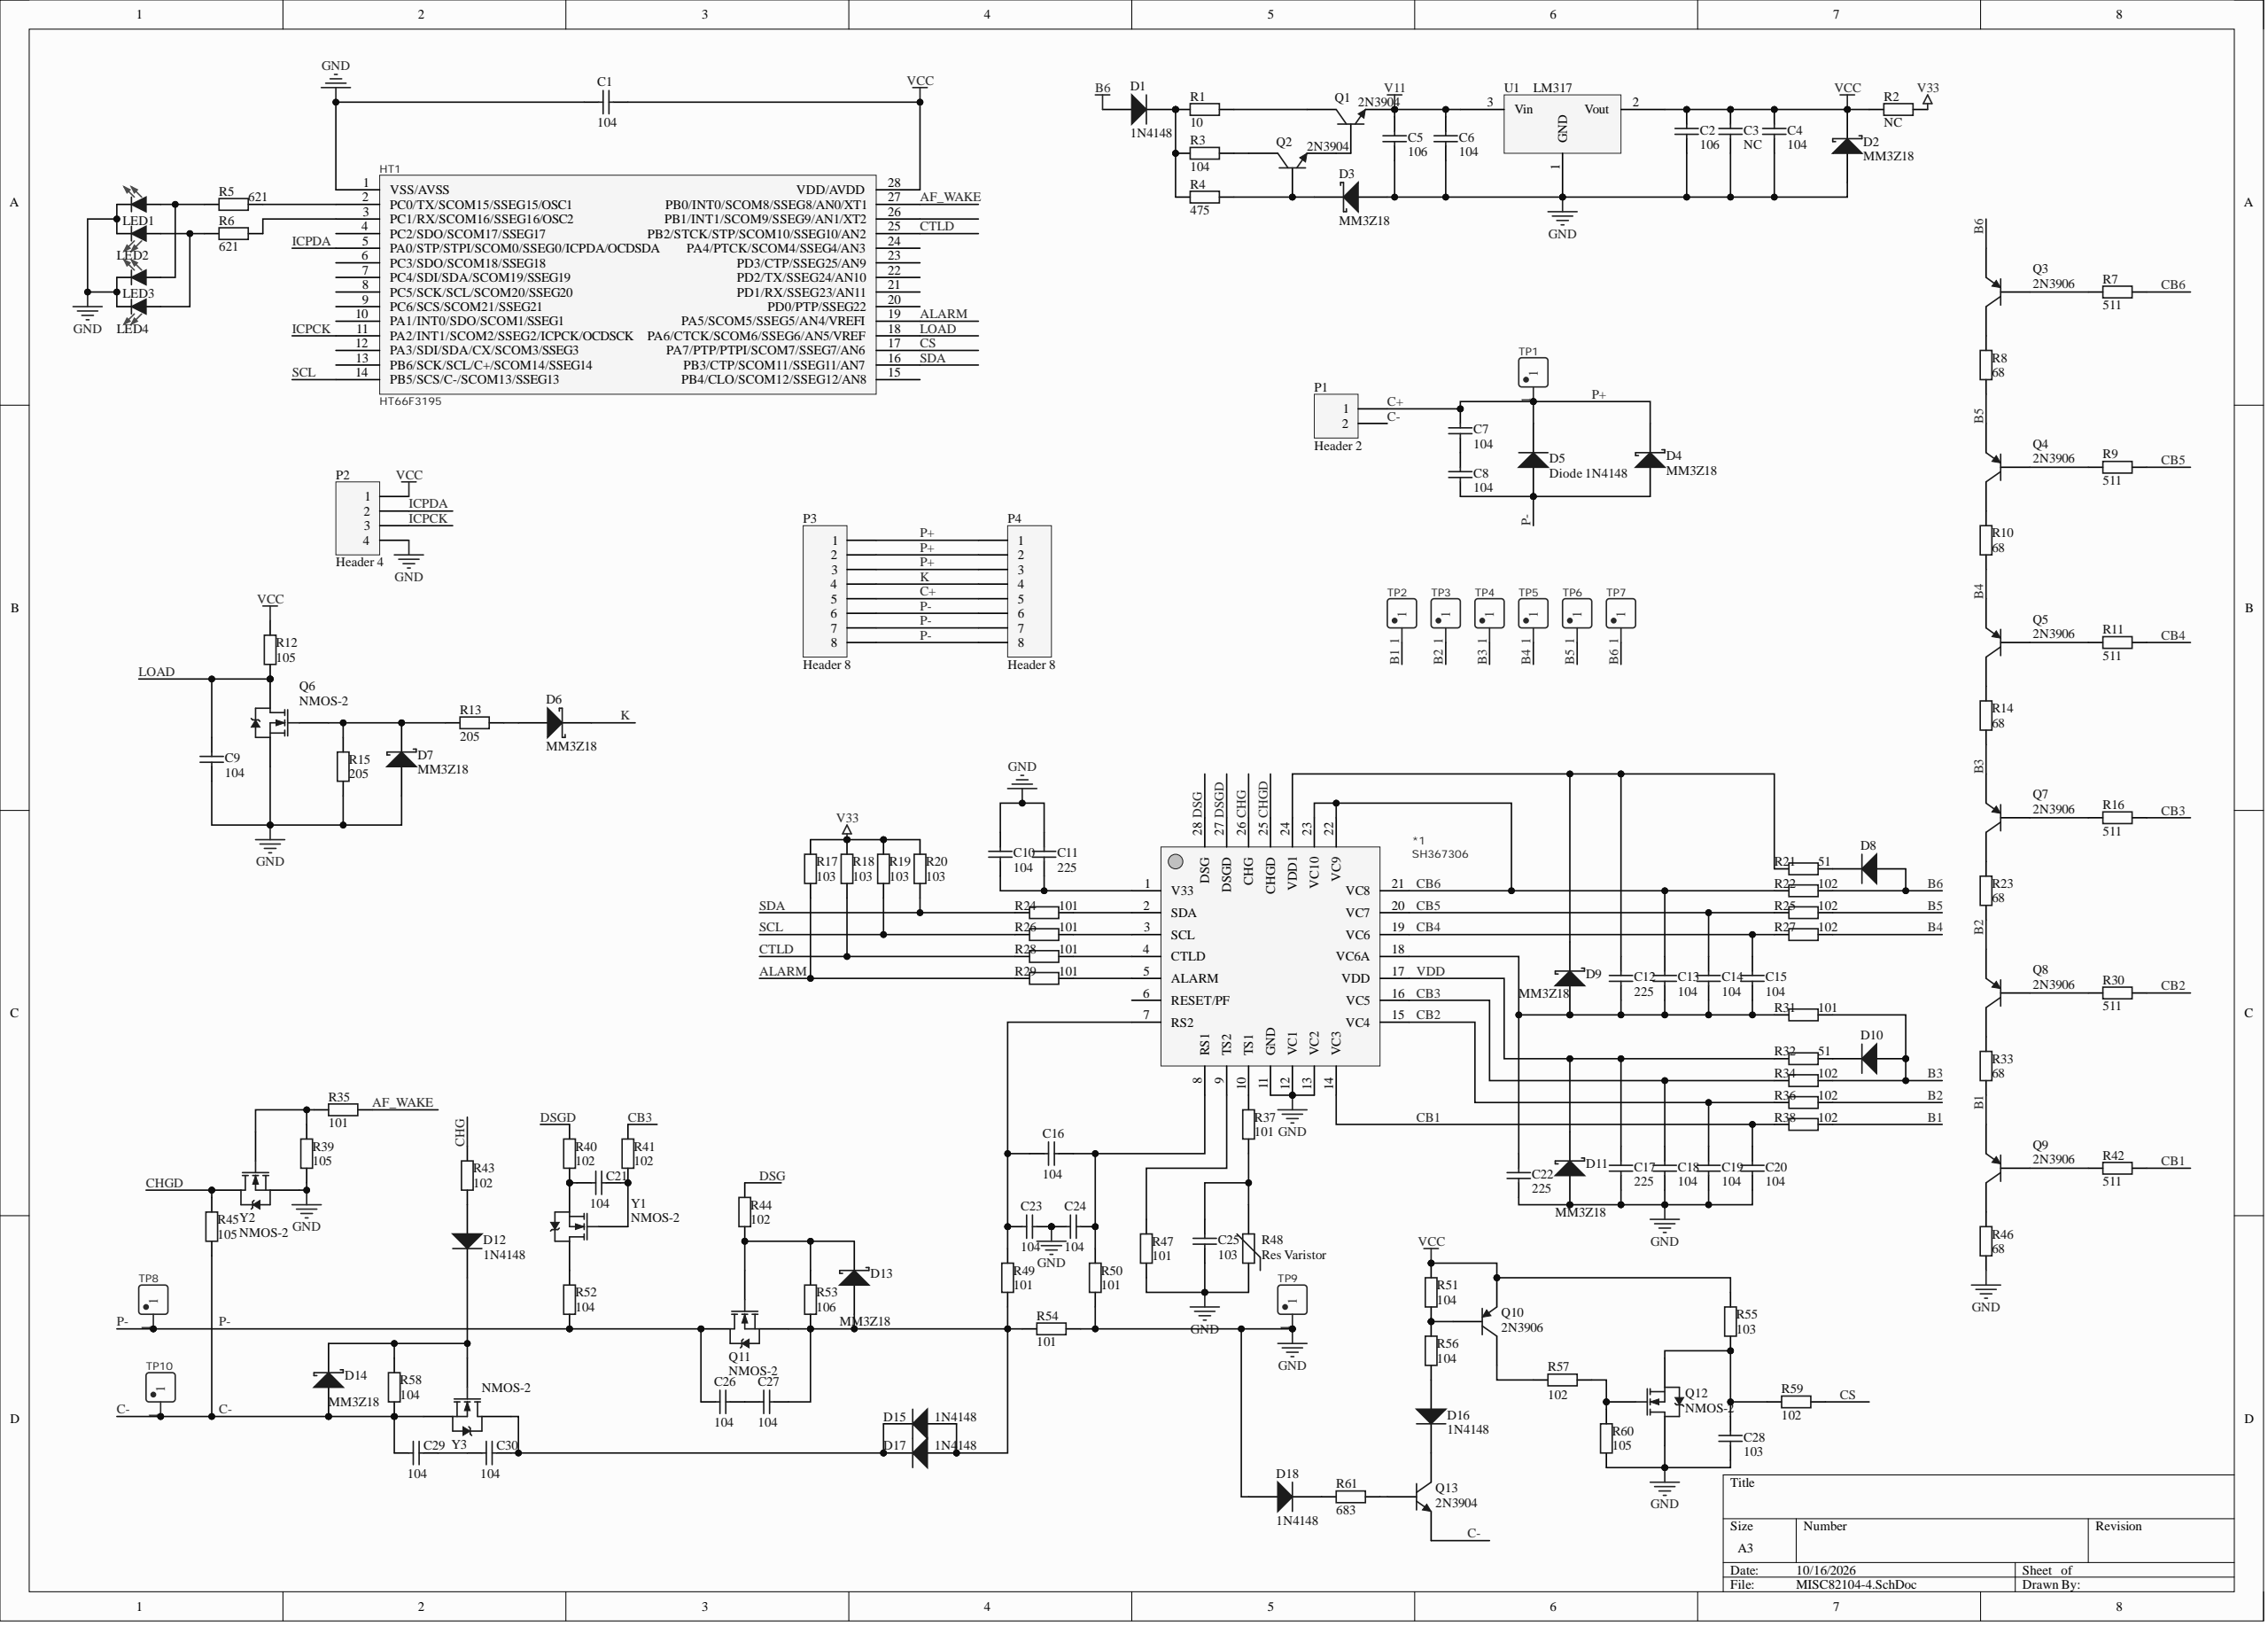Circuit board | Altium Designer | 146 parts | 91 nets
Bill of materials:
Comment,Description,Designator,Footprint,LibRef,Quantity
"SH367306","","*1","QFN28L(5*5)","SH367306","1"
"104","Capacitor","C1, C4, C6, C7, C8, C9, C10, C13, C14, C15, C16, C18, C19, C20, C21, C23, C24, C26, C27, C29, C30","C0603","Cap","21"
"106","Capacitor","C2, C5","C0603","Cap","2"
"NC","Capacitor","C3","C0603","Cap","1"
"225","Capacitor","C11, C12, C17, C22","C0603","Cap","4"
"103","Capacitor","C25, C28","C0603","Cap","2"
"1N4148","High Conductance Fast Diode","D1, D12, D15, D16, D17, D18","DO-35","Diode 1N4148","6"
"MM3Z18","Schottky Rectifier","D2, D3, D4, D6, D7, D9, D11, D13, D14","TO-220AC","Diode 10TQ045","9"
"Diode 1N4148","High Conductance Fast Diode","D5, D8, D10","DO-35","Diode 1N4148","3"
"HT66F3195","","HT1","SSOP28 - DUPLICATE","HT66F3195","1"
"I-LED","Infrared diode","LED1, LED2, LED3, LED4","I-LED-5MM","I-LED","4"
"Header 2","Header, 2-Pin","P1","HDR1X2","Header 2","1"
"Header 4","Header, 4-Pin","P2","HDR1X4","Header 4","1"
"Header 8","Header, 8-Pin","P3, P4","HDR1X8","Header 8","2"
"2N3904","NPN General Purpose Amplifier","Q1, Q2, Q13","TO-92A","2N3904","3"
"2N3906","PNP General Purpose Amplifier","Q3, Q4, Q5, Q7, Q8, Q9, Q10","TO-92A","2N3906","7"
"NMOS-2","N-Channel Power MOSFET","Q6, Q11, Q12, Y1, Y2, Y3","TO-220AB","NMOS-2","6"
"10","Resistor","R1","AXIAL-0.4","Res2","1"
"NC","Resistor","R2","AXIAL-0.4","Res2","1"
"104","Resistor","R3, R51, R52, R56, R58","AXIAL-0.4","Res2","5"
"475","Resistor","R4","AXIAL-0.4","Res2","1"
"621","Resistor","R5, R6","AXIAL-0.4","Res2","2"
"511","Resistor","R7, R9, R11, R16, R30, R42","AXIAL-0.4","Res2","6"
"68","Resistor","R8, R10, R14, R23, R33, R46","AXIAL-0.4","Res2","6"
"105","Resistor","R12, R39, R45, R60","AXIAL-0.4","Res2","4"
"205","Resistor","R13, R15","AXIAL-0.4","Res2","2"
"103","Resistor","R17, R18, R19, R20, R55","AXIAL-0.4","Res2","5"
"51","Resistor","R21, R32","AXIAL-0.4","Res2","2"
"102","Resistor","R22, R25, R27, R34, R36, R38, R40, R41, R43, R44, R57, R59","AXIAL-0.4","Res2","12"
"101","Resistor","R24, R26, R28, R29, R31, R35, R37, R47, R49, R50, R54","AXIAL-0.4","Res2","11"
"Res Varistor","Varistor (Voltage-Sensitive Resistor)","R48","6-0805_N","Res Varistor","1"
"106","Resistor","R53","AXIAL-0.4","Res2","1"
"683","Resistor","R61","AXIAL-0.4","Res2","1"
"TP-RED","","TP1, TP2, TP3, TP4, TP5, TP6, TP7, TP8, TP9, TP10","TEST-TH_BD2.54-P1.4_RED","TP-RED","10"
"LM317","Adjustable linear voltage regulator IC","U1","TO220A","LM317","1"
Netlist (Protel format):
[
*1
QFN28L(5*5)
SH367306



]
[
C1
C0603
104



]
[
C2
C0603
106



]
[
C3
C0603
NC



]
[
C4
C0603
104



]
[
C5
C0603
106



]
[
C6
C0603
104



]
[
C7
C0603
104



]
[
C8
C0603
104



]
[
C9
C0603
104



]
[
C10
C0603
104



]
[
C11
C0603
225



]
[
C12
C0603
225



]
[
C13
C0603
104



]
[
C14
C0603
104



]
[
C15
C0603
104



]
[
C16
C0603
104



]
[
C17
C0603
225



]
[
C18
C0603
104



]
[
C19
C0603
104



]
[
C20
C0603
104



]
[
C21
C0603
104



]
[
C22
C0603
225



]
[
C23
C0603
104



]
[
C24
C0603
104



]
[
C25
C0603
103



]
[
C26
C0603
104



]
[
C27
C0603
104



]
[
C28
C0603
103



]
[
C29
C0603
104



]
[
C30
C0603
104



]
[
D1
DO-35
1N4148



]
[
D2
TO-220AC
MM3Z18



]
[
D3
TO-220AC
MM3Z18



]
[
D4
TO-220AC
MM3Z18



]
[
D5
DO-35
Diode 1N4148



]
[
D6
TO-220AC
MM3Z18



]
[
D7
TO-220AC
MM3Z18



]
[
D8
DO-35
Diode 1N4148



]
[
D9
TO-220AC
MM3Z18



]
[
D10
DO-35
Diode 1N4148



]
[
D11
TO-220AC
MM3Z18



]
[
D12
DO-35
1N4148



]
[
D13
TO-220AC
MM3Z18



]
[
D14
TO-220AC
MM3Z18



]
[
D15
DO-35
1N4148



]
[
D16
DO-35
1N4148



]
[
D17
DO-35
1N4148



]
[
D18
DO-35
1N4148



]
[
HT1
SSOP28 - DUPLICATE
HT66F3195



]
[
LED1
I-LED-5MM
I-LED



]
[
LED2
I-LED-5MM
I-LED



]
[
LED3
I-LED-5MM
I-LED



]
[
LED4
I-LED-5MM
I-LED



]
[
P1
HDR1X2
Header 2



]
[
P2
HDR1X4
Header 4



]
[
P3
HDR1X8
Header 8



]
[
P4
HDR1X8
Header 8



]
[
Q1
TO-92A
2N3904



]
[
Q2
TO-92A
2N3904



]
[
Q3
TO-92A
2N3906



]
[
Q4
TO-92A
2N3906



]
[
Q5
TO-92A
2N3906



]
[
Q6
TO-220AB
NMOS-2



]
[
Q7
TO-92A
2N3906



]
[
Q8
TO-92A
2N3906



]
[
Q9
TO-92A
2N3906



]
[
Q10
TO-92A
2N3906



]
[
Q11
TO-220AB
NMOS-2



]
[
Q12
TO-220AB
NMOS-2



]
[
Q13
TO-92A
2N3904



]
[
R1
AXIAL-0.4
10



]
[
R2
AXIAL-0.4
NC



]
[
R3
AXIAL-0.4
104



]
[
R4
AXIAL-0.4
475



]
[
R5
AXIAL-0.4
621



]
[
R6
AXIAL-0.4
621



]
[
R7
AXIAL-0.4
511



]
[
R8
AXIAL-0.4
68



]
[
R9
AXIAL-0.4
511



]
[
R10
AXIAL-0.4
68



]
[
R11
AXIAL-0.4
511



]
[
R12
AXIAL-0.4
105



]
[
R13
AXIAL-0.4
205



]
[
R14
AXIAL-0.4
68



]
[
R15
AXIAL-0.4
205



]
[
R16
AXIAL-0.4
511



]
[
R17
AXIAL-0.4
103



]
[
R18
AXIAL-0.4
103



]
[
R19
AXIAL-0.4
103



]
[
R20
AXIAL-0.4
103



]
[
R21
AXIAL-0.4
51



]
[
R22
AXIAL-0.4
102



]
[
R23
AXIAL-0.4
68



]
[
R24
AXIAL-0.4
101



]
[
R25
AXIAL-0.4
102



]
[
R26
AXIAL-0.4
101



]
[
R27
AXIAL-0.4
102



]
[
R28
AXIAL-0.4
101



]
[
R29
AXIAL-0.4
101



]
[
R30
AXIAL-0.4
511



]
[
R31
AXIAL-0.4
101



]
[
R32
AXIAL-0.4
51



]
[
R33
AXIAL-0.4
68



]
[
R34
AXIAL-0.4
102



]
[
R35
AXIAL-0.4
101



]
[
R36
AXIAL-0.4
102



]
[
R37
AXIAL-0.4
101



]
[
R38
AXIAL-0.4
102



]
[
R39
AXIAL-0.4
105



]
[
R40
AXIAL-0.4
102



]
[
R41
AXIAL-0.4
102



]
[
R42
AXIAL-0.4
511



]
[
R43
AXIAL-0.4
102



]
[
R44
AXIAL-0.4
102



]
[
R45
AXIAL-0.4
105



]
[
R46
AXIAL-0.4
68



]
[
R47
AXIAL-0.4
101



]
[
R48
6-0805_N
Res Varistor



]
[
R49
AXIAL-0.4
101



]
[
R50
AXIAL-0.4
101



]
[
R51
AXIAL-0.4
104



]
[
R52
AXIAL-0.4
104



]
[
R53
AXIAL-0.4
106



]
[
R54
AXIAL-0.4
101



]
[
R55
AXIAL-0.4
103



]
[
R56
AXIAL-0.4
104



]
[
R57
AXIAL-0.4
102



]
[
R58
AXIAL-0.4
104



]
[
R59
AXIAL-0.4
102



]
[
R60
AXIAL-0.4
105



]
[
R61
AXIAL-0.4
683



]
[
TP1
TEST-TH_BD2.54-P1.4_RED
TP-RED



]
[
TP2
TEST-TH_BD2.54-P1.4_RED
TP-RED



]
[
TP3
TEST-TH_BD2.54-P1.4_RED
TP-RED



]
[
TP4
TEST-TH_BD2.54-P1.4_RED
TP-RED



]
[
TP5
TEST-TH_BD2.54-P1.4_RED
TP-RED



]
[
TP6
TEST-TH_BD2.54-P1.4_RED
TP-RED



]
[
TP7
TEST-TH_BD2.54-P1.4_RED
TP-RED



]
[
TP8
TEST-TH_BD2.54-P1.4_RED
TP-RED



]
[
TP9
TEST-TH_BD2.54-P1.4_RED
TP-RED



]
[
TP10
TEST-TH_BD2.54-P1.4_RED
TP-RED



]
[
U1
TO220A
LM317



]
[
Y1
TO-220AB
NMOS-2



]
[
Y2
TO-220AB
NMOS-2



]
[
Y3
TO-220AB
NMOS-2



]
(
VDD
*1-17
C17-2
D11-1
R32-1
)
(
VCC
C1-2
C2-2
C3-2
C4-2
D2-1
HT1-28
P2-1
Q10-1
R2-1
R12-2
R51-2
R55-1
U1-2
)
(
V33
R2-2
R17-2
R18-2
R19-2
R20-2
)
(
V11
C5-2
C6-2
Q1-1
U1-3
)
(
SDA
HT1-16
R20-1
R24-1
)
(
SCL
HT1-14
R19-1
R26-1
)
(
P-
C8-1
C26-2
D4-3
D5-1
P3-6
P3-7
P3-8
P4-6
P4-7
P4-8
Q11-2
R52-1
TP8-1
)
(
NetR52_2
R52-2
Y1-2
)
(
NetR35_2
R35-2
R39-2
Y2-1
)
(
NetQ13_2
Q13-2
R61-1
)
(
NetQ12_1
Q12-1
R57-1
R60-1
)
(
NetQ10_3
Q10-3
R57-2
)
(
NetQ10_2
Q10-2
R51-1
R56-2
)
(
NetQ9_3
Q9-3
R46-1
)
(
NetQ9_2
Q9-2
R42-2
)
(
NetQ8_3
Q8-3
R33-1
)
(
NetQ8_2
Q8-2
R30-2
)
(
NetQ7_3
Q7-3
R23-1
)
(
NetQ7_2
Q7-2
R16-2
)
(
NetQ5_3
Q5-3
R14-1
)
(
NetQ5_2
Q5-2
R11-2
)
(
NetQ4_3
Q4-3
R10-1
)
(
NetQ4_2
Q4-2
R9-2
)
(
NetQ3_3
Q3-3
R8-1
)
(
NetQ3_2
Q3-2
R7-2
)
(
NetQ2_3
Q2-3
R3-2
)
(
NetQ1_3
Q1-3
R1-2
)
(
NetQ1_2
Q1-2
Q2-1
)
(
NetLED2_1
LED2-1
LED4-1
R6-1
)
(
NetLED1_1
LED1-1
LED3-1
R5-1
)
(
NetHT1_3
HT1-3
R6-2
)
(
NetHT1_2
HT1-2
R5-2
)
(
NetD18_2
D18-2
R61-2
)
(
NetD16_2
D16-2
Q13-3
)
(
NetD16_1
D16-1
R56-1
)
(
NetD13_1
D13-1
Q11-1
R44-1
R53-2
)
(
NetD12_2
D12-2
D14-1
R58-2
Y3-1
)
(
NetD12_1
D12-1
R43-1
)
(
NetD10_2
D10-2
R32-2
)
(
NetD8_2
D8-2
R21-2
)
(
NetD7_1
D7-1
Q6-1
R13-2
R15-2
)
(
NetD6_3
D6-3
R13-1
)
(
NetD3_1
D3-1
Q2-2
R4-2
)
(
NetD1_2
D1-2
R1-1
R3-1
R4-1
)
(
NetC30_1
C30-1
D15-2
D17-2
Y3-2
)
(
NetC29_1
C29-1
C30-2
)
(
NetC28_1
C28-1
Q12-3
R55-2
R59-1
)
(
NetC27_1
C27-1
D13-3
D15-1
D17-1
Q11-3
R49-1
R53-1
R54-2
)
(
NetC26_1
C26-1
C27-2
)
(
NetC25_2
C25-2
R37-1
R48-2
)
(
NetC21_2
C21-2
R40-1
Y1-3
)
(
NetC21_1
C21-1
R41-1
Y1-1
)
(
NetC7_1
C7-1
C8-2
)
(
Net*1_24
*1-24
C12-2
D9-1
R21-1
)
(
Net*1_18
*1-18
C12-1
C13-1
C14-1
C15-1
C22-2
D9-3
R31-1
)
(
Net*1_10
*1-10
R37-2
)
(
Net*1_9
*1-9
R47-2
)
(
Net*1_8
*1-8
C16-1
C24-1
R50-2
)
(
Net*1_7
*1-7
C16-2
C23-2
R49-2
)
(
Net*1_5
*1-5
R29-2
)
(
Net*1_4
*1-4
R28-2
)
(
Net*1_3
*1-3
R26-2
)
(
Net*1_2
*1-2
R24-2
)
(
Net*1_1
*1-1
C10-1
C11-1
)
(
LOAD
C9-2
HT1-18
Q6-2
R12-1
)
(
K
D6-1
P3-4
P4-4
)
(
ICPDA
HT1-5
P2-2
)
(
ICPCK
HT1-11
P2-3
)
(
GND
*1-11
*1-12
*1-13
C1-1
C2-1
C3-1
C4-1
C5-1
C6-1
C9-1
C10-2
C11-2
C17-1
C18-1
C19-1
C20-1
C22-1
C23-1
C24-2
C25-1
C28-2
D2-3
D3-3
D7-3
D11-3
D18-1
HT1-1
LED1-2
LED2-2
LED3-2
LED4-2
P2-4
Q6-3
Q12-2
R15-1
R39-1
R46-2
R47-1
R48-1
R50-1
R54-1
R60-2
TP9-1
U1-1
Y2-3
)
(
DSGD
*1-27
R40-2
)
(
DSG
*1-28
R44-2
)
(
CTLD
HT1-25
R18-1
R28-1
)
(
CS
HT1-17
R59-2
)
(
CHGD
*1-25
R45-2
Y2-2
)
(
CHG
*1-26
R43-2
)
(
CB6
*1-21
*1-22
*1-23
C13-2
R7-1
R22-1
)
(
CB5
*1-20
C14-2
R9-1
R25-1
)
(
CB4
*1-19
C15-2
R11-1
R27-1
)
(
CB3
*1-16
C18-2
R16-1
R34-1
R41-2
)
(
CB2
*1-15
C19-2
R30-1
R36-1
)
(
CB1
*1-14
C20-2
R38-1
R42-1
)
(
C-
C29-2
D14-3
P1-2
Q13-1
R45-1
R58-1
TP10-1
Y3-3
)
(
C+
C7-2
D4-1
D5-2
P1-1
P3-1
P3-2
P3-3
P3-5
P4-1
P4-2
P4-3
P4-5
TP1-1
)
(
B6
D1-1
D8-1
Q3-1
R22-2
TP7-1
)
(
B5
Q4-1
R8-2
R25-2
TP6-1
)
(
B4
Q5-1
R10-2
R27-2
TP5-1
)
(
B3
D10-1
Q7-1
R14-2
R31-2
R34-2
TP4-1
)
(
B2
Q8-1
R23-2
R36-2
TP3-1
)
(
B1
Q9-1
R33-2
R38-2
TP2-1
)
(
ALARM
HT1-19
R17-1
R29-1
)
(
AF_WAKE
HT1-27
R35-1
)